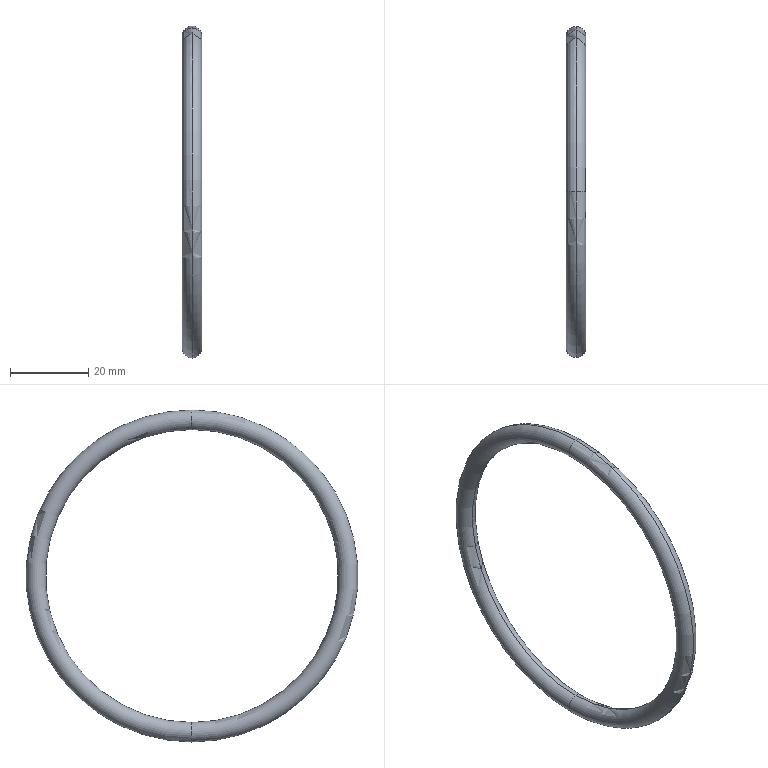Part | SolidWorks | features Revolution 1 | 1 solid | 4 faces | box 5 x 85 x 85 mm | volume 4935 mm3 | torus 4
STEP:
#1=CARTESIAN_POINT('',(0.,0.,-42.5));
#2=VERTEX_POINT('',#1);
#3=CARTESIAN_POINT('',(0.,0.,-37.5));
#4=VERTEX_POINT('',#3);
#5=CARTESIAN_POINT('',(0.,0.,-40.));
#6=DIRECTION('',(0.,1.,0.));
#7=DIRECTION('',(0.,0.,1.));
#8=AXIS2_PLACEMENT_3D('',#5,#6,#7);
#9=CIRCLE('',#8,2.5);
#10=EDGE_CURVE('',#2,#4,#9,.T.);
#11=ORIENTED_EDGE('',*,*,#10,.F.);
#12=CARTESIAN_POINT('',(0.,0.,42.5));
#13=VERTEX_POINT('',#12);
#14=CARTESIAN_POINT('',(0.,0.,0.));
#15=DIRECTION('',(-1.,0.,0.));
#16=DIRECTION('',(0.,0.,1.));
#17=AXIS2_PLACEMENT_3D('',#14,#15,#16);
#18=CIRCLE('',#17,42.5);
#19=EDGE_CURVE('',#2,#13,#18,.T.);
#20=ORIENTED_EDGE('',*,*,#19,.T.);
#21=CARTESIAN_POINT('',(0.,0.,37.5));
#22=VERTEX_POINT('',#21);
#23=CARTESIAN_POINT('',(0.,0.,40.));
#24=DIRECTION('',(0.,-1.,0.));
#25=DIRECTION('',(0.,0.,-1.));
#26=AXIS2_PLACEMENT_3D('',#23,#24,#25);
#27=CIRCLE('',#26,2.5);
#28=EDGE_CURVE('',#13,#22,#27,.T.);
#29=ORIENTED_EDGE('',*,*,#28,.T.);
#30=CARTESIAN_POINT('',(0.,0.,0.));
#31=DIRECTION('',(-1.,0.,0.));
#32=DIRECTION('',(0.,0.,1.));
#33=AXIS2_PLACEMENT_3D('',#30,#31,#32);
#34=CIRCLE('',#33,37.5);
#35=EDGE_CURVE('',#4,#22,#34,.T.);
#36=ORIENTED_EDGE('',*,*,#35,.F.);
#37=EDGE_LOOP('',(#11,#20,#29,#36));
#38=FACE_OUTER_BOUND('',#37,.T.);
#39=CARTESIAN_POINT('',(0.,0.,0.));
#40=DIRECTION('',(-1.,0.,0.));
#41=DIRECTION('',(0.,0.,1.));
#42=AXIS2_PLACEMENT_3D('',#39,#40,#41);
#43=TOROIDAL_SURFACE('',#42,40.,2.5);
#44=ADVANCED_FACE('',(#38),#43,.T.);
#45=ORIENTED_EDGE('',*,*,#28,.F.);
#46=CARTESIAN_POINT('',(0.,0.,0.));
#47=DIRECTION('',(-1.,0.,0.));
#48=DIRECTION('',(0.,0.,1.));
#49=AXIS2_PLACEMENT_3D('',#46,#47,#48);
#50=CIRCLE('',#49,42.5);
#51=EDGE_CURVE('',#13,#2,#50,.T.);
#52=ORIENTED_EDGE('',*,*,#51,.T.);
#53=ORIENTED_EDGE('',*,*,#10,.T.);
#54=CARTESIAN_POINT('',(0.,0.,0.));
#55=DIRECTION('',(-1.,0.,0.));
#56=DIRECTION('',(0.,0.,1.));
#57=AXIS2_PLACEMENT_3D('',#54,#55,#56);
#58=CIRCLE('',#57,37.5);
#59=EDGE_CURVE('',#22,#4,#58,.T.);
#60=ORIENTED_EDGE('',*,*,#59,.F.);
#61=EDGE_LOOP('',(#45,#52,#53,#60));
#62=FACE_OUTER_BOUND('',#61,.T.);
#63=CARTESIAN_POINT('',(0.,0.,0.));
#64=DIRECTION('',(-1.,0.,0.));
#65=DIRECTION('',(0.,0.,1.));
#66=AXIS2_PLACEMENT_3D('',#63,#64,#65);
#67=TOROIDAL_SURFACE('',#66,40.,2.5);
#68=ADVANCED_FACE('',(#62),#67,.T.);
#69=ORIENTED_EDGE('',*,*,#51,.F.);
#70=CARTESIAN_POINT('',(0.,0.,40.));
#71=DIRECTION('',(0.,-1.,0.));
#72=DIRECTION('',(0.,0.,-1.));
#73=AXIS2_PLACEMENT_3D('',#70,#71,#72);
#74=CIRCLE('',#73,2.5);
#75=EDGE_CURVE('',#22,#13,#74,.T.);
#76=ORIENTED_EDGE('',*,*,#75,.F.);
#77=ORIENTED_EDGE('',*,*,#59,.T.);
#78=CARTESIAN_POINT('',(0.,0.,-40.));
#79=DIRECTION('',(0.,1.,0.));
#80=DIRECTION('',(0.,0.,1.));
#81=AXIS2_PLACEMENT_3D('',#78,#79,#80);
#82=CIRCLE('',#81,2.5);
#83=EDGE_CURVE('',#4,#2,#82,.T.);
#84=ORIENTED_EDGE('',*,*,#83,.T.);
#85=EDGE_LOOP('',(#69,#76,#77,#84));
#86=FACE_OUTER_BOUND('',#85,.T.);
#87=CARTESIAN_POINT('',(0.,0.,0.));
#88=DIRECTION('',(-1.,0.,0.));
#89=DIRECTION('',(0.,0.,1.));
#90=AXIS2_PLACEMENT_3D('',#87,#88,#89);
#91=TOROIDAL_SURFACE('',#90,40.,2.5);
#92=ADVANCED_FACE('',(#86),#91,.T.);
#93=ORIENTED_EDGE('',*,*,#19,.F.);
#94=ORIENTED_EDGE('',*,*,#83,.F.);
#95=ORIENTED_EDGE('',*,*,#35,.T.);
#96=ORIENTED_EDGE('',*,*,#75,.T.);
#97=EDGE_LOOP('',(#93,#94,#95,#96));
#98=FACE_OUTER_BOUND('',#97,.T.);
#99=CARTESIAN_POINT('',(0.,0.,0.));
#100=DIRECTION('',(-1.,0.,0.));
#101=DIRECTION('',(0.,0.,1.));
#102=AXIS2_PLACEMENT_3D('',#99,#100,#101);
#103=TOROIDAL_SURFACE('',#102,40.,2.5);
#104=ADVANCED_FACE('',(#98),#103,.T.);
#105=CLOSED_SHELL('',(#44,#68,#92,#104));
#106=MANIFOLD_SOLID_BREP('',#105);
#107=CARTESIAN_POINT('',(0.,0.,0.));
#108=DIRECTION('',(0.,0.,1.));
#109=DIRECTION('',(1.,0.,0.));
#110=AXIS2_PLACEMENT_3D('',#107,#108,#109);
#111=(LENGTH_UNIT()NAMED_UNIT(*)SI_UNIT(.MILLI.,.METRE.));
#112=UNCERTAINTY_MEASURE_WITH_UNIT(LENGTH_MEASURE(0.00001),#111,'','');
#113=(NAMED_UNIT(*)PLANE_ANGLE_UNIT()SI_UNIT($,.RADIAN.));
#114=(NAMED_UNIT(*)SI_UNIT($,.STERADIAN.)SOLID_ANGLE_UNIT());
#115=(GEOMETRIC_REPRESENTATION_CONTEXT(3)GLOBAL_UNCERTAINTY_ASSIGNED_CONTEXT((#112))GLOBAL_UNIT_ASSIGNED_CONTEXT((#111,#113,#114))REPRESENTATION_CONTEXT('',''));
#116=ADVANCED_BREP_SHAPE_REPRESENTATION('',(#106,#110),#115);